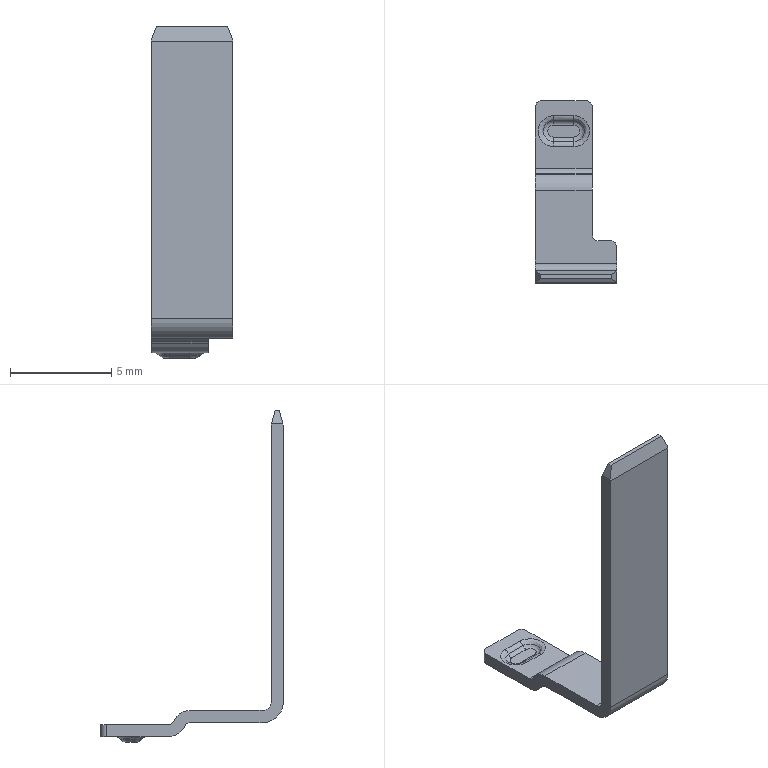Part | STEP file | TQ-DD-1105-THSensorTerminalA1010_デフォルト | 1 solid | 46 faces | box 4 x 9 x 16.36 mm | volume 51.218 mm3 | plane 20 | cylinder 18 | spline 8 | commonest cylinder face diameters 0.6 x10 0.52 x4 1.8 x2 0.8 x1 2 x1